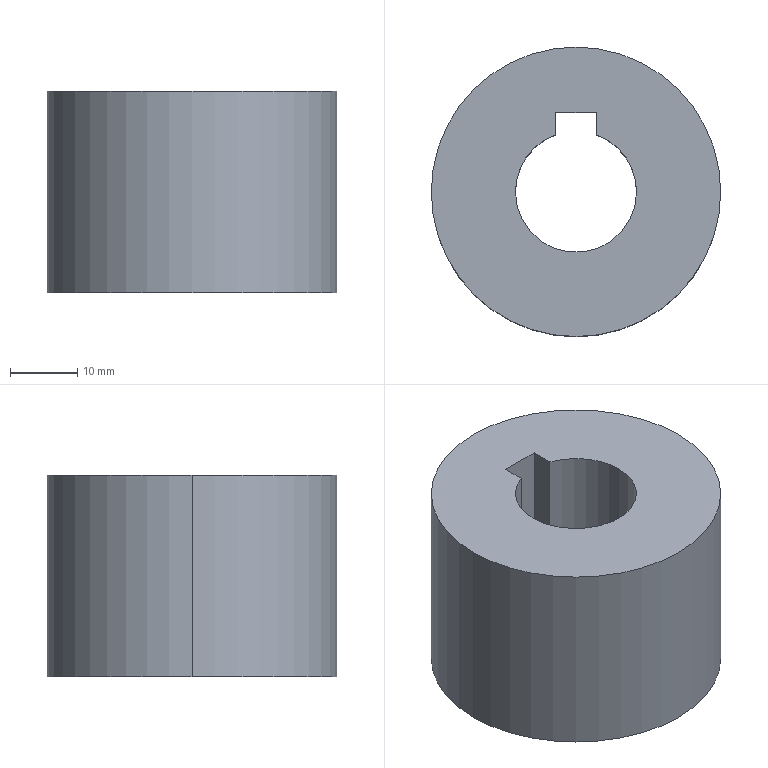Part | SolidWorks | features Extrusion 1, ICE 1 | 1 solid | 10 faces | box 43 x 43 x 30 mm | volume 35397 mm3 | cylinder 5 | plane 5 | commonest cylinder face diameters 18 x3 43 x2
STEP:
#1=CARTESIAN_POINT('',(-9.,0.,-15.));
#2=VERTEX_POINT('',#1);
#3=CARTESIAN_POINT('',(9.,0.,-15.));
#4=VERTEX_POINT('',#3);
#5=CARTESIAN_POINT('',(0.,0.,-15.));
#6=DIRECTION('',(0.,0.,1.));
#7=DIRECTION('',(1.,0.,0.));
#8=AXIS2_PLACEMENT_3D('',#5,#6,#7);
#9=CIRCLE('',#8,9.);
#10=EDGE_CURVE('',#2,#4,#9,.T.);
#11=ORIENTED_EDGE('',*,*,#10,.F.);
#12=CARTESIAN_POINT('',(-9.,0.,15.));
#13=VERTEX_POINT('',#12);
#14=CARTESIAN_POINT('',(-9.,0.,-15.));
#15=DIRECTION('',(0.,0.,1.));
#16=VECTOR('',#15,1000.);
#17=LINE('',#14,#16);
#18=EDGE_CURVE('',#2,#13,#17,.T.);
#19=ORIENTED_EDGE('',*,*,#18,.T.);
#20=CARTESIAN_POINT('',(9.,0.,15.));
#21=VERTEX_POINT('',#20);
#22=CARTESIAN_POINT('',(0.,0.,15.));
#23=DIRECTION('',(0.,0.,1.));
#24=DIRECTION('',(1.,0.,0.));
#25=AXIS2_PLACEMENT_3D('',#22,#23,#24);
#26=CIRCLE('',#25,9.);
#27=EDGE_CURVE('',#13,#21,#26,.T.);
#28=ORIENTED_EDGE('',*,*,#27,.T.);
#29=CARTESIAN_POINT('',(9.,0.,-15.));
#30=DIRECTION('',(0.,0.,1.));
#31=VECTOR('',#30,1000.);
#32=LINE('',#29,#31);
#33=EDGE_CURVE('',#4,#21,#32,.T.);
#34=ORIENTED_EDGE('',*,*,#33,.F.);
#35=EDGE_LOOP('',(#11,#19,#28,#34));
#36=FACE_OUTER_BOUND('',#35,.T.);
#37=CARTESIAN_POINT('',(0.,0.,-15.));
#38=DIRECTION('',(0.,0.,1.));
#39=DIRECTION('',(1.,0.,0.));
#40=AXIS2_PLACEMENT_3D('',#37,#38,#39);
#41=CYLINDRICAL_SURFACE('',#40,9.);
#42=ADVANCED_FACE('',(#36),#41,.F.);
#43=CARTESIAN_POINT('',(3.,8.485,-15.));
#44=VERTEX_POINT('',#43);
#45=CARTESIAN_POINT('',(0.,0.,-15.));
#46=DIRECTION('',(0.,0.,1.));
#47=DIRECTION('',(1.,0.,0.));
#48=AXIS2_PLACEMENT_3D('',#45,#46,#47);
#49=CIRCLE('',#48,9.);
#50=EDGE_CURVE('',#4,#44,#49,.T.);
#51=ORIENTED_EDGE('',*,*,#50,.F.);
#52=ORIENTED_EDGE('',*,*,#33,.T.);
#53=CARTESIAN_POINT('',(3.,8.485,15.));
#54=VERTEX_POINT('',#53);
#55=CARTESIAN_POINT('',(0.,0.,15.));
#56=DIRECTION('',(0.,0.,1.));
#57=DIRECTION('',(1.,0.,0.));
#58=AXIS2_PLACEMENT_3D('',#55,#56,#57);
#59=CIRCLE('',#58,9.);
#60=EDGE_CURVE('',#21,#54,#59,.T.);
#61=ORIENTED_EDGE('',*,*,#60,.T.);
#62=CARTESIAN_POINT('',(3.,8.485,-15.));
#63=DIRECTION('',(0.,0.,1.));
#64=VECTOR('',#63,1000.);
#65=LINE('',#62,#64);
#66=EDGE_CURVE('',#44,#54,#65,.T.);
#67=ORIENTED_EDGE('',*,*,#66,.F.);
#68=EDGE_LOOP('',(#51,#52,#61,#67));
#69=FACE_OUTER_BOUND('',#68,.T.);
#70=CARTESIAN_POINT('',(0.,0.,-15.));
#71=DIRECTION('',(0.,0.,1.));
#72=DIRECTION('',(1.,0.,0.));
#73=AXIS2_PLACEMENT_3D('',#70,#71,#72);
#74=CYLINDRICAL_SURFACE('',#73,9.);
#75=ADVANCED_FACE('',(#69),#74,.F.);
#76=CARTESIAN_POINT('',(21.5,0.,15.));
#77=VERTEX_POINT('',#76);
#78=CARTESIAN_POINT('',(-21.5,0.,15.));
#79=VERTEX_POINT('',#78);
#80=CARTESIAN_POINT('',(0.,0.,15.));
#81=DIRECTION('',(0.,0.,1.));
#82=DIRECTION('',(1.,0.,0.));
#83=AXIS2_PLACEMENT_3D('',#80,#81,#82);
#84=CIRCLE('',#83,21.5);
#85=EDGE_CURVE('',#77,#79,#84,.T.);
#86=ORIENTED_EDGE('',*,*,#85,.F.);
#87=CARTESIAN_POINT('',(21.5,0.,-15.));
#88=VERTEX_POINT('',#87);
#89=CARTESIAN_POINT('',(21.5,0.,15.));
#90=DIRECTION('',(0.,0.,-1.));
#91=VECTOR('',#90,1000.);
#92=LINE('',#89,#91);
#93=EDGE_CURVE('',#77,#88,#92,.T.);
#94=ORIENTED_EDGE('',*,*,#93,.T.);
#95=CARTESIAN_POINT('',(-21.5,0.,-15.));
#96=VERTEX_POINT('',#95);
#97=CARTESIAN_POINT('',(0.,0.,-15.));
#98=DIRECTION('',(0.,0.,1.));
#99=DIRECTION('',(1.,0.,0.));
#100=AXIS2_PLACEMENT_3D('',#97,#98,#99);
#101=CIRCLE('',#100,21.5);
#102=EDGE_CURVE('',#88,#96,#101,.T.);
#103=ORIENTED_EDGE('',*,*,#102,.T.);
#104=CARTESIAN_POINT('',(-21.5,0.,15.));
#105=DIRECTION('',(0.,0.,-1.));
#106=VECTOR('',#105,1000.);
#107=LINE('',#104,#106);
#108=EDGE_CURVE('',#79,#96,#107,.T.);
#109=ORIENTED_EDGE('',*,*,#108,.F.);
#110=EDGE_LOOP('',(#86,#94,#103,#109));
#111=FACE_OUTER_BOUND('',#110,.T.);
#112=CARTESIAN_POINT('',(0.,0.,15.));
#113=DIRECTION('',(0.,0.,-1.));
#114=DIRECTION('',(-1.,0.,0.));
#115=AXIS2_PLACEMENT_3D('',#112,#113,#114);
#116=CYLINDRICAL_SURFACE('',#115,21.5);
#117=ADVANCED_FACE('',(#111),#116,.T.);
#118=ORIENTED_EDGE('',*,*,#93,.F.);
#119=CARTESIAN_POINT('',(0.,0.,15.));
#120=DIRECTION('',(0.,0.,1.));
#121=DIRECTION('',(1.,0.,0.));
#122=AXIS2_PLACEMENT_3D('',#119,#120,#121);
#123=CIRCLE('',#122,21.5);
#124=EDGE_CURVE('',#79,#77,#123,.T.);
#125=ORIENTED_EDGE('',*,*,#124,.F.);
#126=ORIENTED_EDGE('',*,*,#108,.T.);
#127=CARTESIAN_POINT('',(0.,0.,-15.));
#128=DIRECTION('',(0.,0.,1.));
#129=DIRECTION('',(1.,0.,0.));
#130=AXIS2_PLACEMENT_3D('',#127,#128,#129);
#131=CIRCLE('',#130,21.5);
#132=EDGE_CURVE('',#96,#88,#131,.T.);
#133=ORIENTED_EDGE('',*,*,#132,.T.);
#134=EDGE_LOOP('',(#118,#125,#126,#133));
#135=FACE_OUTER_BOUND('',#134,.T.);
#136=CARTESIAN_POINT('',(0.,0.,15.));
#137=DIRECTION('',(0.,0.,-1.));
#138=DIRECTION('',(-1.,0.,0.));
#139=AXIS2_PLACEMENT_3D('',#136,#137,#138);
#140=CYLINDRICAL_SURFACE('',#139,21.5);
#141=ADVANCED_FACE('',(#135),#140,.T.);
#142=CARTESIAN_POINT('',(-3.,8.485,15.));
#143=VERTEX_POINT('',#142);
#144=CARTESIAN_POINT('',(0.,0.,15.));
#145=DIRECTION('',(0.,0.,1.));
#146=DIRECTION('',(1.,0.,0.));
#147=AXIS2_PLACEMENT_3D('',#144,#145,#146);
#148=CIRCLE('',#147,9.);
#149=EDGE_CURVE('',#143,#13,#148,.T.);
#150=ORIENTED_EDGE('',*,*,#149,.F.);
#151=CARTESIAN_POINT('',(-3.,11.8,15.));
#152=VERTEX_POINT('',#151);
#153=CARTESIAN_POINT('',(-3.,11.8,15.));
#154=DIRECTION('',(0.,-1.,0.));
#155=VECTOR('',#154,1000.);
#156=LINE('',#153,#155);
#157=EDGE_CURVE('',#152,#143,#156,.T.);
#158=ORIENTED_EDGE('',*,*,#157,.F.);
#159=CARTESIAN_POINT('',(3.,11.8,15.));
#160=VERTEX_POINT('',#159);
#161=CARTESIAN_POINT('',(-3.,11.8,15.));
#162=DIRECTION('',(-1.,0.,0.));
#163=VECTOR('',#162,1000.);
#164=LINE('',#161,#163);
#165=EDGE_CURVE('',#160,#152,#164,.T.);
#166=ORIENTED_EDGE('',*,*,#165,.F.);
#167=CARTESIAN_POINT('',(3.,11.8,15.));
#168=DIRECTION('',(0.,1.,0.));
#169=VECTOR('',#168,1000.);
#170=LINE('',#167,#169);
#171=EDGE_CURVE('',#54,#160,#170,.T.);
#172=ORIENTED_EDGE('',*,*,#171,.F.);
#173=ORIENTED_EDGE('',*,*,#60,.F.);
#174=ORIENTED_EDGE('',*,*,#27,.F.);
#175=EDGE_LOOP('',(#150,#158,#166,#172,#173,#174));
#176=FACE_BOUND('',#175,.T.);
#177=ORIENTED_EDGE('',*,*,#124,.T.);
#178=ORIENTED_EDGE('',*,*,#85,.T.);
#179=EDGE_LOOP('',(#177,#178));
#180=FACE_OUTER_BOUND('',#179,.T.);
#181=CARTESIAN_POINT('',(0.,0.,15.));
#182=DIRECTION('',(0.,0.,1.));
#183=DIRECTION('',(1.,0.,0.));
#184=AXIS2_PLACEMENT_3D('',#181,#182,#183);
#185=PLANE('',#184);
#186=ADVANCED_FACE('',(#176,#180),#185,.T.);
#187=CARTESIAN_POINT('',(-3.,11.8,-15.));
#188=VERTEX_POINT('',#187);
#189=CARTESIAN_POINT('',(-3.,8.485,-15.));
#190=VERTEX_POINT('',#189);
#191=CARTESIAN_POINT('',(-3.,11.8,-15.));
#192=DIRECTION('',(0.,-1.,0.));
#193=VECTOR('',#192,1000.);
#194=LINE('',#191,#193);
#195=EDGE_CURVE('',#188,#190,#194,.T.);
#196=ORIENTED_EDGE('',*,*,#195,.T.);
#197=CARTESIAN_POINT('',(0.,0.,-15.));
#198=DIRECTION('',(0.,0.,1.));
#199=DIRECTION('',(1.,0.,0.));
#200=AXIS2_PLACEMENT_3D('',#197,#198,#199);
#201=CIRCLE('',#200,9.);
#202=EDGE_CURVE('',#190,#2,#201,.T.);
#203=ORIENTED_EDGE('',*,*,#202,.T.);
#204=ORIENTED_EDGE('',*,*,#10,.T.);
#205=ORIENTED_EDGE('',*,*,#50,.T.);
#206=CARTESIAN_POINT('',(3.,11.8,-15.));
#207=VERTEX_POINT('',#206);
#208=CARTESIAN_POINT('',(3.,11.8,-15.));
#209=DIRECTION('',(0.,1.,0.));
#210=VECTOR('',#209,1000.);
#211=LINE('',#208,#210);
#212=EDGE_CURVE('',#44,#207,#211,.T.);
#213=ORIENTED_EDGE('',*,*,#212,.T.);
#214=CARTESIAN_POINT('',(-3.,11.8,-15.));
#215=DIRECTION('',(-1.,0.,0.));
#216=VECTOR('',#215,1000.);
#217=LINE('',#214,#216);
#218=EDGE_CURVE('',#207,#188,#217,.T.);
#219=ORIENTED_EDGE('',*,*,#218,.T.);
#220=EDGE_LOOP('',(#196,#203,#204,#205,#213,#219));
#221=FACE_BOUND('',#220,.T.);
#222=ORIENTED_EDGE('',*,*,#132,.F.);
#223=ORIENTED_EDGE('',*,*,#102,.F.);
#224=EDGE_LOOP('',(#222,#223));
#225=FACE_OUTER_BOUND('',#224,.T.);
#226=CARTESIAN_POINT('',(0.,0.,-15.));
#227=DIRECTION('',(0.,0.,1.));
#228=DIRECTION('',(1.,0.,0.));
#229=AXIS2_PLACEMENT_3D('',#226,#227,#228);
#230=PLANE('',#229);
#231=ADVANCED_FACE('',(#221,#225),#230,.F.);
#232=ORIENTED_EDGE('',*,*,#18,.F.);
#233=ORIENTED_EDGE('',*,*,#202,.F.);
#234=CARTESIAN_POINT('',(-3.,8.485,-15.));
#235=DIRECTION('',(0.,0.,1.));
#236=VECTOR('',#235,1000.);
#237=LINE('',#234,#236);
#238=EDGE_CURVE('',#190,#143,#237,.T.);
#239=ORIENTED_EDGE('',*,*,#238,.T.);
#240=ORIENTED_EDGE('',*,*,#149,.T.);
#241=EDGE_LOOP('',(#232,#233,#239,#240));
#242=FACE_OUTER_BOUND('',#241,.T.);
#243=CARTESIAN_POINT('',(0.,0.,-15.));
#244=DIRECTION('',(0.,0.,1.));
#245=DIRECTION('',(1.,0.,0.));
#246=AXIS2_PLACEMENT_3D('',#243,#244,#245);
#247=CYLINDRICAL_SURFACE('',#246,9.);
#248=ADVANCED_FACE('',(#242),#247,.F.);
#249=ORIENTED_EDGE('',*,*,#157,.T.);
#250=ORIENTED_EDGE('',*,*,#238,.F.);
#251=ORIENTED_EDGE('',*,*,#195,.F.);
#252=CARTESIAN_POINT('',(-3.,11.8,-15.));
#253=DIRECTION('',(0.,0.,1.));
#254=VECTOR('',#253,1000.);
#255=LINE('',#252,#254);
#256=EDGE_CURVE('',#188,#152,#255,.T.);
#257=ORIENTED_EDGE('',*,*,#256,.T.);
#258=EDGE_LOOP('',(#249,#250,#251,#257));
#259=FACE_OUTER_BOUND('',#258,.T.);
#260=CARTESIAN_POINT('',(-3.,11.8,-15.));
#261=DIRECTION('',(-1.,0.,0.));
#262=DIRECTION('',(0.,-1.,0.));
#263=AXIS2_PLACEMENT_3D('',#260,#261,#262);
#264=PLANE('',#263);
#265=ADVANCED_FACE('',(#259),#264,.F.);
#266=ORIENTED_EDGE('',*,*,#165,.T.);
#267=ORIENTED_EDGE('',*,*,#256,.F.);
#268=ORIENTED_EDGE('',*,*,#218,.F.);
#269=CARTESIAN_POINT('',(3.,11.8,-15.));
#270=DIRECTION('',(0.,0.,1.));
#271=VECTOR('',#270,1000.);
#272=LINE('',#269,#271);
#273=EDGE_CURVE('',#207,#160,#272,.T.);
#274=ORIENTED_EDGE('',*,*,#273,.T.);
#275=EDGE_LOOP('',(#266,#267,#268,#274));
#276=FACE_OUTER_BOUND('',#275,.T.);
#277=CARTESIAN_POINT('',(-3.,11.8,-15.));
#278=DIRECTION('',(0.,1.,0.));
#279=DIRECTION('',(0.,0.,1.));
#280=AXIS2_PLACEMENT_3D('',#277,#278,#279);
#281=PLANE('',#280);
#282=ADVANCED_FACE('',(#276),#281,.F.);
#283=ORIENTED_EDGE('',*,*,#171,.T.);
#284=ORIENTED_EDGE('',*,*,#273,.F.);
#285=ORIENTED_EDGE('',*,*,#212,.F.);
#286=ORIENTED_EDGE('',*,*,#66,.T.);
#287=EDGE_LOOP('',(#283,#284,#285,#286));
#288=FACE_OUTER_BOUND('',#287,.T.);
#289=CARTESIAN_POINT('',(3.,11.8,-15.));
#290=DIRECTION('',(1.,0.,0.));
#291=DIRECTION('',(0.,1.,0.));
#292=AXIS2_PLACEMENT_3D('',#289,#290,#291);
#293=PLANE('',#292);
#294=ADVANCED_FACE('',(#288),#293,.F.);
#295=CLOSED_SHELL('',(#42,#75,#117,#141,#186,#231,#248,#265,#282,#294));
#296=MANIFOLD_SOLID_BREP('',#295);
#297=CARTESIAN_POINT('',(0.,0.,0.));
#298=DIRECTION('',(0.,0.,1.));
#299=DIRECTION('',(1.,0.,0.));
#300=AXIS2_PLACEMENT_3D('',#297,#298,#299);
#301=(LENGTH_UNIT()NAMED_UNIT(*)SI_UNIT(.MILLI.,.METRE.));
#302=UNCERTAINTY_MEASURE_WITH_UNIT(LENGTH_MEASURE(0.00001),#301,'','');
#303=(NAMED_UNIT(*)PLANE_ANGLE_UNIT()SI_UNIT($,.RADIAN.));
#304=(NAMED_UNIT(*)SI_UNIT($,.STERADIAN.)SOLID_ANGLE_UNIT());
#305=(GEOMETRIC_REPRESENTATION_CONTEXT(3)GLOBAL_UNCERTAINTY_ASSIGNED_CONTEXT((#302))GLOBAL_UNIT_ASSIGNED_CONTEXT((#301,#303,#304))REPRESENTATION_CONTEXT('',''));
#306=ADVANCED_BREP_SHAPE_REPRESENTATION('',(#296,#300),#305);